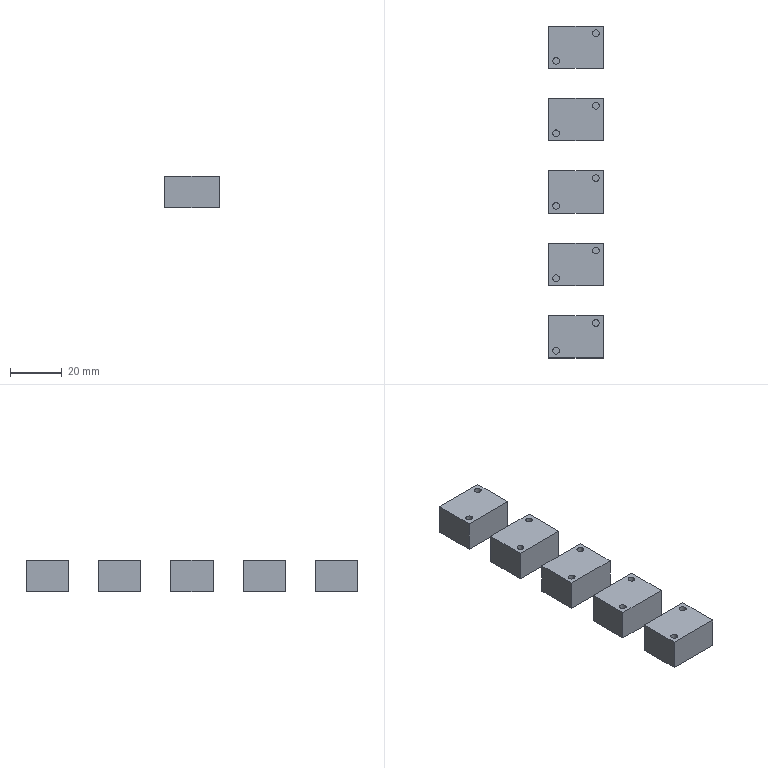Part | 5 solids | 60 faces | box 21 x 128.262 x 12 mm | volume 20066 mm3 | plane 40 | cylinder 20 | commonest cylinder face diameters 2.6 x20
STEP:
#1=CARTESIAN_POINT('',(-10.5,-47.869,0.));
#2=VERTEX_POINT('',#1);
#3=CARTESIAN_POINT('',(-10.5,-64.131,0.));
#4=VERTEX_POINT('',#3);
#5=CARTESIAN_POINT('',(-10.5,-47.869,0.));
#6=DIRECTION('',(0.,-1.,0.));
#7=VECTOR('',#6,1000.);
#8=LINE('',#5,#7);
#9=EDGE_CURVE('',#2,#4,#8,.T.);
#10=ORIENTED_EDGE('',*,*,#9,.T.);
#11=CARTESIAN_POINT('',(10.5,-64.131,0.));
#12=VERTEX_POINT('',#11);
#13=CARTESIAN_POINT('',(-10.5,-64.131,0.));
#14=DIRECTION('',(1.,0.,0.));
#15=VECTOR('',#14,1000.);
#16=LINE('',#13,#15);
#17=EDGE_CURVE('',#4,#12,#16,.T.);
#18=ORIENTED_EDGE('',*,*,#17,.T.);
#19=CARTESIAN_POINT('',(10.5,-47.869,0.));
#20=VERTEX_POINT('',#19);
#21=CARTESIAN_POINT('',(10.5,-64.131,0.));
#22=DIRECTION('',(0.,1.,0.));
#23=VECTOR('',#22,1000.);
#24=LINE('',#21,#23);
#25=EDGE_CURVE('',#12,#20,#24,.T.);
#26=ORIENTED_EDGE('',*,*,#25,.T.);
#27=CARTESIAN_POINT('',(10.5,-47.869,0.));
#28=DIRECTION('',(-1.,0.,0.));
#29=VECTOR('',#28,1000.);
#30=LINE('',#27,#29);
#31=EDGE_CURVE('',#20,#2,#30,.T.);
#32=ORIENTED_EDGE('',*,*,#31,.T.);
#33=EDGE_LOOP('',(#10,#18,#26,#32));
#34=FACE_BOUND('',#33,.T.);
#35=CARTESIAN_POINT('',(9.,-50.669,0.));
#36=VERTEX_POINT('',#35);
#37=CARTESIAN_POINT('',(6.4,-50.669,0.));
#38=VERTEX_POINT('',#37);
#39=CARTESIAN_POINT('',(7.7,-50.669,0.));
#40=DIRECTION('',(0.,0.,-1.));
#41=DIRECTION('',(1.,0.,0.));
#42=AXIS2_PLACEMENT_3D('',#39,#40,#41);
#43=CIRCLE('',#42,1.3);
#44=EDGE_CURVE('',#36,#38,#43,.T.);
#45=ORIENTED_EDGE('',*,*,#44,.T.);
#46=CARTESIAN_POINT('',(7.7,-50.669,0.));
#47=DIRECTION('',(0.,0.,-1.));
#48=DIRECTION('',(-1.,0.,0.));
#49=AXIS2_PLACEMENT_3D('',#46,#47,#48);
#50=CIRCLE('',#49,1.3);
#51=EDGE_CURVE('',#38,#36,#50,.T.);
#52=ORIENTED_EDGE('',*,*,#51,.T.);
#53=EDGE_LOOP('',(#45,#52));
#54=FACE_BOUND('',#53,.T.);
#55=CARTESIAN_POINT('',(-6.4,-61.331,0.));
#56=VERTEX_POINT('',#55);
#57=CARTESIAN_POINT('',(-9.,-61.331,0.));
#58=VERTEX_POINT('',#57);
#59=CARTESIAN_POINT('',(-7.7,-61.331,0.));
#60=DIRECTION('',(0.,0.,-1.));
#61=DIRECTION('',(1.,0.,0.));
#62=AXIS2_PLACEMENT_3D('',#59,#60,#61);
#63=CIRCLE('',#62,1.3);
#64=EDGE_CURVE('',#56,#58,#63,.T.);
#65=ORIENTED_EDGE('',*,*,#64,.T.);
#66=CARTESIAN_POINT('',(-7.7,-61.331,0.));
#67=DIRECTION('',(0.,0.,-1.));
#68=DIRECTION('',(-1.,0.,0.));
#69=AXIS2_PLACEMENT_3D('',#66,#67,#68);
#70=CIRCLE('',#69,1.3);
#71=EDGE_CURVE('',#58,#56,#70,.T.);
#72=ORIENTED_EDGE('',*,*,#71,.T.);
#73=EDGE_LOOP('',(#65,#72));
#74=FACE_BOUND('',#73,.T.);
#75=CARTESIAN_POINT('',(13.231,-129.333,0.));
#76=DIRECTION('',(0.,0.,-1.));
#77=DIRECTION('',(1.,0.,0.));
#78=AXIS2_PLACEMENT_3D('',#75,#76,#77);
#79=PLANE('',#78);
#80=ADVANCED_FACE('',(#34,#54,#74),#79,.F.);
#81=ORIENTED_EDGE('',*,*,#31,.F.);
#82=CARTESIAN_POINT('',(10.5,-47.869,-12.));
#83=VERTEX_POINT('',#82);
#84=CARTESIAN_POINT('',(10.5,-47.869,0.));
#85=DIRECTION('',(0.,0.,-1.));
#86=VECTOR('',#85,1000.);
#87=LINE('',#84,#86);
#88=EDGE_CURVE('',#20,#83,#87,.T.);
#89=ORIENTED_EDGE('',*,*,#88,.T.);
#90=CARTESIAN_POINT('',(-10.5,-47.869,-12.));
#91=VERTEX_POINT('',#90);
#92=CARTESIAN_POINT('',(10.5,-47.869,-12.));
#93=DIRECTION('',(-1.,0.,0.));
#94=VECTOR('',#93,1000.);
#95=LINE('',#92,#94);
#96=EDGE_CURVE('',#83,#91,#95,.T.);
#97=ORIENTED_EDGE('',*,*,#96,.T.);
#98=CARTESIAN_POINT('',(-10.5,-47.869,0.));
#99=DIRECTION('',(0.,0.,-1.));
#100=VECTOR('',#99,1000.);
#101=LINE('',#98,#100);
#102=EDGE_CURVE('',#2,#91,#101,.T.);
#103=ORIENTED_EDGE('',*,*,#102,.F.);
#104=EDGE_LOOP('',(#81,#89,#97,#103));
#105=FACE_BOUND('',#104,.T.);
#106=CARTESIAN_POINT('',(13.231,-47.869,0.));
#107=DIRECTION('',(0.,-1.,0.));
#108=DIRECTION('',(1.,0.,0.));
#109=AXIS2_PLACEMENT_3D('',#106,#107,#108);
#110=PLANE('',#109);
#111=ADVANCED_FACE('',(#105),#110,.F.);
#112=CARTESIAN_POINT('',(-10.5,-64.131,-12.));
#113=VERTEX_POINT('',#112);
#114=CARTESIAN_POINT('',(-10.5,-64.131,-12.));
#115=DIRECTION('',(0.,1.,0.));
#116=VECTOR('',#115,1000.);
#117=LINE('',#114,#116);
#118=EDGE_CURVE('',#113,#91,#117,.T.);
#119=ORIENTED_EDGE('',*,*,#118,.F.);
#120=CARTESIAN_POINT('',(-10.5,-64.131,-12.));
#121=DIRECTION('',(0.,0.,1.));
#122=VECTOR('',#121,1000.);
#123=LINE('',#120,#122);
#124=EDGE_CURVE('',#113,#4,#123,.T.);
#125=ORIENTED_EDGE('',*,*,#124,.T.);
#126=ORIENTED_EDGE('',*,*,#9,.F.);
#127=ORIENTED_EDGE('',*,*,#102,.T.);
#128=EDGE_LOOP('',(#119,#125,#126,#127));
#129=FACE_BOUND('',#128,.T.);
#130=CARTESIAN_POINT('',(-10.5,-64.131,0.));
#131=DIRECTION('',(-1.,0.,0.));
#132=DIRECTION('',(0.,-1.,0.));
#133=AXIS2_PLACEMENT_3D('',#130,#131,#132);
#134=PLANE('',#133);
#135=ADVANCED_FACE('',(#129),#134,.T.);
#136=ORIENTED_EDGE('',*,*,#124,.F.);
#137=CARTESIAN_POINT('',(10.5,-64.131,-12.));
#138=VERTEX_POINT('',#137);
#139=CARTESIAN_POINT('',(10.5,-64.131,-12.));
#140=DIRECTION('',(-1.,0.,0.));
#141=VECTOR('',#140,1000.);
#142=LINE('',#139,#141);
#143=EDGE_CURVE('',#138,#113,#142,.T.);
#144=ORIENTED_EDGE('',*,*,#143,.F.);
#145=CARTESIAN_POINT('',(10.5,-64.131,-12.));
#146=DIRECTION('',(0.,0.,1.));
#147=VECTOR('',#146,1000.);
#148=LINE('',#145,#147);
#149=EDGE_CURVE('',#138,#12,#148,.T.);
#150=ORIENTED_EDGE('',*,*,#149,.T.);
#151=ORIENTED_EDGE('',*,*,#17,.F.);
#152=EDGE_LOOP('',(#136,#144,#150,#151));
#153=FACE_BOUND('',#152,.T.);
#154=CARTESIAN_POINT('',(10.5,-64.131,0.));
#155=DIRECTION('',(0.,-1.,0.));
#156=DIRECTION('',(1.,0.,0.));
#157=AXIS2_PLACEMENT_3D('',#154,#155,#156);
#158=PLANE('',#157);
#159=ADVANCED_FACE('',(#153),#158,.T.);
#160=ORIENTED_EDGE('',*,*,#25,.F.);
#161=ORIENTED_EDGE('',*,*,#149,.F.);
#162=CARTESIAN_POINT('',(10.5,-47.869,-12.));
#163=DIRECTION('',(0.,-1.,0.));
#164=VECTOR('',#163,1000.);
#165=LINE('',#162,#164);
#166=EDGE_CURVE('',#83,#138,#165,.T.);
#167=ORIENTED_EDGE('',*,*,#166,.F.);
#168=ORIENTED_EDGE('',*,*,#88,.F.);
#169=EDGE_LOOP('',(#160,#161,#167,#168));
#170=FACE_BOUND('',#169,.T.);
#171=CARTESIAN_POINT('',(10.5,-43.561,0.));
#172=DIRECTION('',(1.,0.,0.));
#173=DIRECTION('',(0.,1.,0.));
#174=AXIS2_PLACEMENT_3D('',#171,#172,#173);
#175=PLANE('',#174);
#176=ADVANCED_FACE('',(#170),#175,.T.);
#177=ORIENTED_EDGE('',*,*,#166,.T.);
#178=ORIENTED_EDGE('',*,*,#143,.T.);
#179=ORIENTED_EDGE('',*,*,#118,.T.);
#180=ORIENTED_EDGE('',*,*,#96,.F.);
#181=EDGE_LOOP('',(#177,#178,#179,#180));
#182=FACE_BOUND('',#181,.T.);
#183=CARTESIAN_POINT('',(18.713,-139.577,-12.));
#184=DIRECTION('',(0.,0.,-1.));
#185=DIRECTION('',(1.,0.,0.));
#186=AXIS2_PLACEMENT_3D('',#183,#184,#185);
#187=PLANE('',#186);
#188=ADVANCED_FACE('',(#182),#187,.T.);
#189=CARTESIAN_POINT('',(6.4,-50.669,-8.));
#190=VERTEX_POINT('',#189);
#191=CARTESIAN_POINT('',(6.4,-50.669,0.));
#192=DIRECTION('',(0.,0.,-1.));
#193=VECTOR('',#192,1000.);
#194=LINE('',#191,#193);
#195=EDGE_CURVE('',#190,#38,#194,.F.);
#196=ORIENTED_EDGE('',*,*,#195,.F.);
#197=CARTESIAN_POINT('',(9.,-50.669,-8.));
#198=VERTEX_POINT('',#197);
#199=CARTESIAN_POINT('',(7.7,-50.669,-8.));
#200=DIRECTION('',(0.,0.,-1.));
#201=DIRECTION('',(-1.,0.,0.));
#202=AXIS2_PLACEMENT_3D('',#199,#200,#201);
#203=CIRCLE('',#202,1.3);
#204=EDGE_CURVE('',#190,#198,#203,.T.);
#205=ORIENTED_EDGE('',*,*,#204,.T.);
#206=CARTESIAN_POINT('',(9.,-50.669,0.));
#207=DIRECTION('',(0.,0.,-1.));
#208=VECTOR('',#207,1000.);
#209=LINE('',#206,#208);
#210=EDGE_CURVE('',#198,#36,#209,.F.);
#211=ORIENTED_EDGE('',*,*,#210,.T.);
#212=ORIENTED_EDGE('',*,*,#51,.F.);
#213=EDGE_LOOP('',(#196,#205,#211,#212));
#214=FACE_BOUND('',#213,.T.);
#215=CARTESIAN_POINT('',(7.7,-50.669,0.));
#216=DIRECTION('',(0.,0.,-1.));
#217=DIRECTION('',(1.,0.,0.));
#218=AXIS2_PLACEMENT_3D('',#215,#216,#217);
#219=CYLINDRICAL_SURFACE('',#218,1.3);
#220=ADVANCED_FACE('',(#214),#219,.F.);
#221=ORIENTED_EDGE('',*,*,#210,.F.);
#222=CARTESIAN_POINT('',(7.7,-50.669,-8.));
#223=DIRECTION('',(0.,0.,-1.));
#224=DIRECTION('',(1.,0.,0.));
#225=AXIS2_PLACEMENT_3D('',#222,#223,#224);
#226=CIRCLE('',#225,1.3);
#227=EDGE_CURVE('',#198,#190,#226,.T.);
#228=ORIENTED_EDGE('',*,*,#227,.T.);
#229=ORIENTED_EDGE('',*,*,#195,.T.);
#230=ORIENTED_EDGE('',*,*,#44,.F.);
#231=EDGE_LOOP('',(#221,#228,#229,#230));
#232=FACE_BOUND('',#231,.T.);
#233=CARTESIAN_POINT('',(7.7,-50.669,0.));
#234=DIRECTION('',(0.,0.,-1.));
#235=DIRECTION('',(1.,0.,0.));
#236=AXIS2_PLACEMENT_3D('',#233,#234,#235);
#237=CYLINDRICAL_SURFACE('',#236,1.3);
#238=ADVANCED_FACE('',(#232),#237,.F.);
#239=ORIENTED_EDGE('',*,*,#227,.F.);
#240=ORIENTED_EDGE('',*,*,#204,.F.);
#241=EDGE_LOOP('',(#239,#240));
#242=FACE_BOUND('',#241,.T.);
#243=CARTESIAN_POINT('',(13.231,-129.333,-8.));
#244=DIRECTION('',(0.,0.,-1.));
#245=DIRECTION('',(1.,0.,0.));
#246=AXIS2_PLACEMENT_3D('',#243,#244,#245);
#247=PLANE('',#246);
#248=ADVANCED_FACE('',(#242),#247,.F.);
#249=CARTESIAN_POINT('',(-6.4,-61.331,-8.));
#250=VERTEX_POINT('',#249);
#251=CARTESIAN_POINT('',(-9.,-61.331,-8.));
#252=VERTEX_POINT('',#251);
#253=CARTESIAN_POINT('',(-7.7,-61.331,-8.));
#254=DIRECTION('',(0.,0.,-1.));
#255=DIRECTION('',(1.,0.,0.));
#256=AXIS2_PLACEMENT_3D('',#253,#254,#255);
#257=CIRCLE('',#256,1.3);
#258=EDGE_CURVE('',#250,#252,#257,.T.);
#259=ORIENTED_EDGE('',*,*,#258,.F.);
#260=CARTESIAN_POINT('',(-7.7,-61.331,-8.));
#261=DIRECTION('',(0.,0.,-1.));
#262=DIRECTION('',(-1.,0.,0.));
#263=AXIS2_PLACEMENT_3D('',#260,#261,#262);
#264=CIRCLE('',#263,1.3);
#265=EDGE_CURVE('',#252,#250,#264,.T.);
#266=ORIENTED_EDGE('',*,*,#265,.F.);
#267=EDGE_LOOP('',(#259,#266));
#268=FACE_BOUND('',#267,.T.);
#269=CARTESIAN_POINT('',(13.231,-129.333,-8.));
#270=DIRECTION('',(0.,0.,-1.));
#271=DIRECTION('',(1.,0.,0.));
#272=AXIS2_PLACEMENT_3D('',#269,#270,#271);
#273=PLANE('',#272);
#274=ADVANCED_FACE('',(#268),#273,.F.);
#275=CARTESIAN_POINT('',(-9.,-61.331,0.));
#276=DIRECTION('',(0.,0.,-1.));
#277=VECTOR('',#276,1000.);
#278=LINE('',#275,#277);
#279=EDGE_CURVE('',#252,#58,#278,.F.);
#280=ORIENTED_EDGE('',*,*,#279,.F.);
#281=ORIENTED_EDGE('',*,*,#265,.T.);
#282=CARTESIAN_POINT('',(-6.4,-61.331,0.));
#283=DIRECTION('',(0.,0.,-1.));
#284=VECTOR('',#283,1000.);
#285=LINE('',#282,#284);
#286=EDGE_CURVE('',#250,#56,#285,.F.);
#287=ORIENTED_EDGE('',*,*,#286,.T.);
#288=ORIENTED_EDGE('',*,*,#71,.F.);
#289=EDGE_LOOP('',(#280,#281,#287,#288));
#290=FACE_BOUND('',#289,.T.);
#291=CARTESIAN_POINT('',(-7.7,-61.331,0.));
#292=DIRECTION('',(0.,0.,-1.));
#293=DIRECTION('',(1.,0.,0.));
#294=AXIS2_PLACEMENT_3D('',#291,#292,#293);
#295=CYLINDRICAL_SURFACE('',#294,1.3);
#296=ADVANCED_FACE('',(#290),#295,.F.);
#297=ORIENTED_EDGE('',*,*,#286,.F.);
#298=ORIENTED_EDGE('',*,*,#258,.T.);
#299=ORIENTED_EDGE('',*,*,#279,.T.);
#300=ORIENTED_EDGE('',*,*,#64,.F.);
#301=EDGE_LOOP('',(#297,#298,#299,#300));
#302=FACE_BOUND('',#301,.T.);
#303=CARTESIAN_POINT('',(-7.7,-61.331,0.));
#304=DIRECTION('',(0.,0.,-1.));
#305=DIRECTION('',(1.,0.,0.));
#306=AXIS2_PLACEMENT_3D('',#303,#304,#305);
#307=CYLINDRICAL_SURFACE('',#306,1.3);
#308=ADVANCED_FACE('',(#302),#307,.F.);
#309=CLOSED_SHELL('',(#80,#111,#135,#159,#176,#188,#220,#238,#248,#274,#296,#308));
#310=MANIFOLD_SOLID_BREP('',#309);
#311=CARTESIAN_POINT('',(-10.5,-19.869,0.));
#312=VERTEX_POINT('',#311);
#313=CARTESIAN_POINT('',(-10.5,-36.131,0.));
#314=VERTEX_POINT('',#313);
#315=CARTESIAN_POINT('',(-10.5,-19.869,0.));
#316=DIRECTION('',(0.,-1.,0.));
#317=VECTOR('',#316,1000.);
#318=LINE('',#315,#317);
#319=EDGE_CURVE('',#312,#314,#318,.T.);
#320=ORIENTED_EDGE('',*,*,#319,.T.);
#321=CARTESIAN_POINT('',(10.5,-36.131,0.));
#322=VERTEX_POINT('',#321);
#323=CARTESIAN_POINT('',(-10.5,-36.131,0.));
#324=DIRECTION('',(1.,0.,0.));
#325=VECTOR('',#324,1000.);
#326=LINE('',#323,#325);
#327=EDGE_CURVE('',#314,#322,#326,.T.);
#328=ORIENTED_EDGE('',*,*,#327,.T.);
#329=CARTESIAN_POINT('',(10.5,-19.869,0.));
#330=VERTEX_POINT('',#329);
#331=CARTESIAN_POINT('',(10.5,-36.131,0.));
#332=DIRECTION('',(0.,1.,0.));
#333=VECTOR('',#332,1000.);
#334=LINE('',#331,#333);
#335=EDGE_CURVE('',#322,#330,#334,.T.);
#336=ORIENTED_EDGE('',*,*,#335,.T.);
#337=CARTESIAN_POINT('',(10.5,-19.869,0.));
#338=DIRECTION('',(-1.,0.,0.));
#339=VECTOR('',#338,1000.);
#340=LINE('',#337,#339);
#341=EDGE_CURVE('',#330,#312,#340,.T.);
#342=ORIENTED_EDGE('',*,*,#341,.T.);
#343=EDGE_LOOP('',(#320,#328,#336,#342));
#344=FACE_BOUND('',#343,.T.);
#345=CARTESIAN_POINT('',(9.,-22.669,0.));
#346=VERTEX_POINT('',#345);
#347=CARTESIAN_POINT('',(6.4,-22.669,0.));
#348=VERTEX_POINT('',#347);
#349=CARTESIAN_POINT('',(7.7,-22.669,0.));
#350=DIRECTION('',(0.,0.,-1.));
#351=DIRECTION('',(1.,0.,0.));
#352=AXIS2_PLACEMENT_3D('',#349,#350,#351);
#353=CIRCLE('',#352,1.3);
#354=EDGE_CURVE('',#346,#348,#353,.T.);
#355=ORIENTED_EDGE('',*,*,#354,.T.);
#356=CARTESIAN_POINT('',(7.7,-22.669,0.));
#357=DIRECTION('',(0.,0.,-1.));
#358=DIRECTION('',(-1.,0.,0.));
#359=AXIS2_PLACEMENT_3D('',#356,#357,#358);
#360=CIRCLE('',#359,1.3);
#361=EDGE_CURVE('',#348,#346,#360,.T.);
#362=ORIENTED_EDGE('',*,*,#361,.T.);
#363=EDGE_LOOP('',(#355,#362));
#364=FACE_BOUND('',#363,.T.);
#365=CARTESIAN_POINT('',(-6.4,-33.331,0.));
#366=VERTEX_POINT('',#365);
#367=CARTESIAN_POINT('',(-9.,-33.331,0.));
#368=VERTEX_POINT('',#367);
#369=CARTESIAN_POINT('',(-7.7,-33.331,0.));
#370=DIRECTION('',(0.,0.,-1.));
#371=DIRECTION('',(1.,0.,0.));
#372=AXIS2_PLACEMENT_3D('',#369,#370,#371);
#373=CIRCLE('',#372,1.3);
#374=EDGE_CURVE('',#366,#368,#373,.T.);
#375=ORIENTED_EDGE('',*,*,#374,.T.);
#376=CARTESIAN_POINT('',(-7.7,-33.331,0.));
#377=DIRECTION('',(0.,0.,-1.));
#378=DIRECTION('',(-1.,0.,0.));
#379=AXIS2_PLACEMENT_3D('',#376,#377,#378);
#380=CIRCLE('',#379,1.3);
#381=EDGE_CURVE('',#368,#366,#380,.T.);
#382=ORIENTED_EDGE('',*,*,#381,.T.);
#383=EDGE_LOOP('',(#375,#382));
#384=FACE_BOUND('',#383,.T.);
#385=CARTESIAN_POINT('',(13.231,-101.333,0.));
#386=DIRECTION('',(0.,0.,-1.));
#387=DIRECTION('',(1.,0.,0.));
#388=AXIS2_PLACEMENT_3D('',#385,#386,#387);
#389=PLANE('',#388);
#390=ADVANCED_FACE('',(#344,#364,#384),#389,.F.);
#391=ORIENTED_EDGE('',*,*,#341,.F.);
#392=CARTESIAN_POINT('',(10.5,-19.869,-12.));
#393=VERTEX_POINT('',#392);
#394=CARTESIAN_POINT('',(10.5,-19.869,0.));
#395=DIRECTION('',(0.,0.,-1.));
#396=VECTOR('',#395,1000.);
#397=LINE('',#394,#396);
#398=EDGE_CURVE('',#330,#393,#397,.T.);
#399=ORIENTED_EDGE('',*,*,#398,.T.);
#400=CARTESIAN_POINT('',(-10.5,-19.869,-12.));
#401=VERTEX_POINT('',#400);
#402=CARTESIAN_POINT('',(10.5,-19.869,-12.));
#403=DIRECTION('',(-1.,0.,0.));
#404=VECTOR('',#403,1000.);
#405=LINE('',#402,#404);
#406=EDGE_CURVE('',#393,#401,#405,.T.);
#407=ORIENTED_EDGE('',*,*,#406,.T.);
#408=CARTESIAN_POINT('',(-10.5,-19.869,0.));
#409=DIRECTION('',(0.,0.,-1.));
#410=VECTOR('',#409,1000.);
#411=LINE('',#408,#410);
#412=EDGE_CURVE('',#312,#401,#411,.T.);
#413=ORIENTED_EDGE('',*,*,#412,.F.);
#414=EDGE_LOOP('',(#391,#399,#407,#413));
#415=FACE_BOUND('',#414,.T.);
#416=CARTESIAN_POINT('',(13.231,-19.869,0.));
#417=DIRECTION('',(0.,-1.,0.));
#418=DIRECTION('',(1.,0.,0.));
#419=AXIS2_PLACEMENT_3D('',#416,#417,#418);
#420=PLANE('',#419);
#421=ADVANCED_FACE('',(#415),#420,.F.);
#422=CARTESIAN_POINT('',(-10.5,-36.131,-12.));
#423=VERTEX_POINT('',#422);
#424=CARTESIAN_POINT('',(-10.5,-36.131,-12.));
#425=DIRECTION('',(0.,1.,0.));
#426=VECTOR('',#425,1000.);
#427=LINE('',#424,#426);
#428=EDGE_CURVE('',#423,#401,#427,.T.);
#429=ORIENTED_EDGE('',*,*,#428,.F.);
#430=CARTESIAN_POINT('',(-10.5,-36.131,-12.));
#431=DIRECTION('',(0.,0.,1.));
#432=VECTOR('',#431,1000.);
#433=LINE('',#430,#432);
#434=EDGE_CURVE('',#423,#314,#433,.T.);
#435=ORIENTED_EDGE('',*,*,#434,.T.);
#436=ORIENTED_EDGE('',*,*,#319,.F.);
#437=ORIENTED_EDGE('',*,*,#412,.T.);
#438=EDGE_LOOP('',(#429,#435,#436,#437));
#439=FACE_BOUND('',#438,.T.);
#440=CARTESIAN_POINT('',(-10.5,-36.131,0.));
#441=DIRECTION('',(-1.,0.,0.));
#442=DIRECTION('',(0.,-1.,0.));
#443=AXIS2_PLACEMENT_3D('',#440,#441,#442);
#444=PLANE('',#443);
#445=ADVANCED_FACE('',(#439),#444,.T.);
#446=ORIENTED_EDGE('',*,*,#434,.F.);
#447=CARTESIAN_POINT('',(10.5,-36.131,-12.));
#448=VERTEX_POINT('',#447);
#449=CARTESIAN_POINT('',(10.5,-36.131,-12.));
#450=DIRECTION('',(-1.,0.,0.));
#451=VECTOR('',#450,1000.);
#452=LINE('',#449,#451);
#453=EDGE_CURVE('',#448,#423,#452,.T.);
#454=ORIENTED_EDGE('',*,*,#453,.F.);
#455=CARTESIAN_POINT('',(10.5,-36.131,-12.));
#456=DIRECTION('',(0.,0.,1.));
#457=VECTOR('',#456,1000.);
#458=LINE('',#455,#457);
#459=EDGE_CURVE('',#448,#322,#458,.T.);
#460=ORIENTED_EDGE('',*,*,#459,.T.);
#461=ORIENTED_EDGE('',*,*,#327,.F.);
#462=EDGE_LOOP('',(#446,#454,#460,#461));
#463=FACE_BOUND('',#462,.T.);
#464=CARTESIAN_POINT('',(10.5,-36.131,0.));
#465=DIRECTION('',(0.,-1.,0.));
#466=DIRECTION('',(1.,0.,0.));
#467=AXIS2_PLACEMENT_3D('',#464,#465,#466);
#468=PLANE('',#467);
#469=ADVANCED_FACE('',(#463),#468,.T.);
#470=ORIENTED_EDGE('',*,*,#335,.F.);
#471=ORIENTED_EDGE('',*,*,#459,.F.);
#472=CARTESIAN_POINT('',(10.5,-19.869,-12.));
#473=DIRECTION('',(0.,-1.,0.));
#474=VECTOR('',#473,1000.);
#475=LINE('',#472,#474);
#476=EDGE_CURVE('',#393,#448,#475,.T.);
#477=ORIENTED_EDGE('',*,*,#476,.F.);
#478=ORIENTED_EDGE('',*,*,#398,.F.);
#479=EDGE_LOOP('',(#470,#471,#477,#478));
#480=FACE_BOUND('',#479,.T.);
#481=CARTESIAN_POINT('',(10.5,-15.561,0.));
#482=DIRECTION('',(1.,0.,0.));
#483=DIRECTION('',(0.,1.,0.));
#484=AXIS2_PLACEMENT_3D('',#481,#482,#483);
#485=PLANE('',#484);
#486=ADVANCED_FACE('',(#480),#485,.T.);
#487=ORIENTED_EDGE('',*,*,#476,.T.);
#488=ORIENTED_EDGE('',*,*,#453,.T.);
#489=ORIENTED_EDGE('',*,*,#428,.T.);
#490=ORIENTED_EDGE('',*,*,#406,.F.);
#491=EDGE_LOOP('',(#487,#488,#489,#490));
#492=FACE_BOUND('',#491,.T.);
#493=CARTESIAN_POINT('',(18.713,-111.577,-12.));
#494=DIRECTION('',(0.,0.,-1.));
#495=DIRECTION('',(1.,0.,0.));
#496=AXIS2_PLACEMENT_3D('',#493,#494,#495);
#497=PLANE('',#496);
#498=ADVANCED_FACE('',(#492),#497,.T.);
#499=CARTESIAN_POINT('',(6.4,-22.669,-8.));
#500=VERTEX_POINT('',#499);
#501=CARTESIAN_POINT('',(6.4,-22.669,0.));
#502=DIRECTION('',(0.,0.,-1.));
#503=VECTOR('',#502,1000.);
#504=LINE('',#501,#503);
#505=EDGE_CURVE('',#500,#348,#504,.F.);
#506=ORIENTED_EDGE('',*,*,#505,.F.);
#507=CARTESIAN_POINT('',(9.,-22.669,-8.));
#508=VERTEX_POINT('',#507);
#509=CARTESIAN_POINT('',(7.7,-22.669,-8.));
#510=DIRECTION('',(0.,0.,-1.));
#511=DIRECTION('',(-1.,0.,0.));
#512=AXIS2_PLACEMENT_3D('',#509,#510,#511);
#513=CIRCLE('',#512,1.3);
#514=EDGE_CURVE('',#500,#508,#513,.T.);
#515=ORIENTED_EDGE('',*,*,#514,.T.);
#516=CARTESIAN_POINT('',(9.,-22.669,0.));
#517=DIRECTION('',(0.,0.,-1.));
#518=VECTOR('',#517,1000.);
#519=LINE('',#516,#518);
#520=EDGE_CURVE('',#508,#346,#519,.F.);
#521=ORIENTED_EDGE('',*,*,#520,.T.);
#522=ORIENTED_EDGE('',*,*,#361,.F.);
#523=EDGE_LOOP('',(#506,#515,#521,#522));
#524=FACE_BOUND('',#523,.T.);
#525=CARTESIAN_POINT('',(7.7,-22.669,0.));
#526=DIRECTION('',(0.,0.,-1.));
#527=DIRECTION('',(1.,0.,0.));
#528=AXIS2_PLACEMENT_3D('',#525,#526,#527);
#529=CYLINDRICAL_SURFACE('',#528,1.3);
#530=ADVANCED_FACE('',(#524),#529,.F.);
#531=ORIENTED_EDGE('',*,*,#520,.F.);
#532=CARTESIAN_POINT('',(7.7,-22.669,-8.));
#533=DIRECTION('',(0.,0.,-1.));
#534=DIRECTION('',(1.,0.,0.));
#535=AXIS2_PLACEMENT_3D('',#532,#533,#534);
#536=CIRCLE('',#535,1.3);
#537=EDGE_CURVE('',#508,#500,#536,.T.);
#538=ORIENTED_EDGE('',*,*,#537,.T.);
#539=ORIENTED_EDGE('',*,*,#505,.T.);
#540=ORIENTED_EDGE('',*,*,#354,.F.);
#541=EDGE_LOOP('',(#531,#538,#539,#540));
#542=FACE_BOUND('',#541,.T.);
#543=CARTESIAN_POINT('',(7.7,-22.669,0.));
#544=DIRECTION('',(0.,0.,-1.));
#545=DIRECTION('',(1.,0.,0.));
#546=AXIS2_PLACEMENT_3D('',#543,#544,#545);
#547=CYLINDRICAL_SURFACE('',#546,1.3);
#548=ADVANCED_FACE('',(#542),#547,.F.);
#549=ORIENTED_EDGE('',*,*,#537,.F.);
#550=ORIENTED_EDGE('',*,*,#514,.F.);
#551=EDGE_LOOP('',(#549,#550));
#552=FACE_BOUND('',#551,.T.);
#553=CARTESIAN_POINT('',(13.231,-101.333,-8.));
#554=DIRECTION('',(0.,0.,-1.));
#555=DIRECTION('',(1.,0.,0.));
#556=AXIS2_PLACEMENT_3D('',#553,#554,#555);
#557=PLANE('',#556);
#558=ADVANCED_FACE('',(#552),#557,.F.);
#559=CARTESIAN_POINT('',(-6.4,-33.331,-8.));
#560=VERTEX_POINT('',#559);
#561=CARTESIAN_POINT('',(-9.,-33.331,-8.));
#562=VERTEX_POINT('',#561);
#563=CARTESIAN_POINT('',(-7.7,-33.331,-8.));
#564=DIRECTION('',(0.,0.,-1.));
#565=DIRECTION('',(1.,0.,0.));
#566=AXIS2_PLACEMENT_3D('',#563,#564,#565);
#567=CIRCLE('',#566,1.3);
#568=EDGE_CURVE('',#560,#562,#567,.T.);
#569=ORIENTED_EDGE('',*,*,#568,.F.);
#570=CARTESIAN_POINT('',(-7.7,-33.331,-8.));
#571=DIRECTION('',(0.,0.,-1.));
#572=DIRECTION('',(-1.,0.,0.));
#573=AXIS2_PLACEMENT_3D('',#570,#571,#572);
#574=CIRCLE('',#573,1.3);
#575=EDGE_CURVE('',#562,#560,#574,.T.);
#576=ORIENTED_EDGE('',*,*,#575,.F.);
#577=EDGE_LOOP('',(#569,#576));
#578=FACE_BOUND('',#577,.T.);
#579=CARTESIAN_POINT('',(13.231,-101.333,-8.));
#580=DIRECTION('',(0.,0.,-1.));
#581=DIRECTION('',(1.,0.,0.));
#582=AXIS2_PLACEMENT_3D('',#579,#580,#581);
#583=PLANE('',#582);
#584=ADVANCED_FACE('',(#578),#583,.F.);
#585=CARTESIAN_POINT('',(-9.,-33.331,0.));
#586=DIRECTION('',(0.,0.,-1.));
#587=VECTOR('',#586,1000.);
#588=LINE('',#585,#587);
#589=EDGE_CURVE('',#562,#368,#588,.F.);
#590=ORIENTED_EDGE('',*,*,#589,.F.);
#591=ORIENTED_EDGE('',*,*,#575,.T.);
#592=CARTESIAN_POINT('',(-6.4,-33.331,0.));
#593=DIRECTION('',(0.,0.,-1.));
#594=VECTOR('',#593,1000.);
#595=LINE('',#592,#594);
#596=EDGE_CURVE('',#560,#366,#595,.F.);
#597=ORIENTED_EDGE('',*,*,#596,.T.);
#598=ORIENTED_EDGE('',*,*,#381,.F.);
#599=EDGE_LOOP('',(#590,#591,#597,#598));
#600=FACE_BOUND('',#599,.T.);
#601=CARTESIAN_POINT('',(-7.7,-33.331,0.));
#602=DIRECTION('',(0.,0.,-1.));
#603=DIRECTION('',(1.,0.,0.));
#604=AXIS2_PLACEMENT_3D('',#601,#602,#603);
#605=CYLINDRICAL_SURFACE('',#604,1.3);
#606=ADVANCED_FACE('',(#600),#605,.F.);
#607=ORIENTED_EDGE('',*,*,#596,.F.);
#608=ORIENTED_EDGE('',*,*,#568,.T.);
#609=ORIENTED_EDGE('',*,*,#589,.T.);
#610=ORIENTED_EDGE('',*,*,#374,.F.);
#611=EDGE_LOOP('',(#607,#608,#609,#610));
#612=FACE_BOUND('',#611,.T.);
#613=CARTESIAN_POINT('',(-7.7,-33.331,0.));
#614=DIRECTION('',(0.,0.,-1.));
#615=DIRECTION('',(1.,0.,0.));
#616=AXIS2_PLACEMENT_3D('',#613,#614,#615);
#617=CYLINDRICAL_SURFACE('',#616,1.3);
#618=ADVANCED_FACE('',(#612),#617,.F.);
#619=CLOSED_SHELL('',(#390,#421,#445,#469,#486,#498,#530,#548,#558,#584,#606,#618));
#620=MANIFOLD_SOLID_BREP('',#619);
#621=CARTESIAN_POINT('',(-10.5,-103.869,0.));
#622=VERTEX_POINT('',#621);
#623=CARTESIAN_POINT('',(-10.5,-120.131,0.));
#624=VERTEX_POINT('',#623);
#625=CARTESIAN_POINT('',(-10.5,-103.869,0.));
#626=DIRECTION('',(0.,-1.,0.));
#627=VECTOR('',#626,1000.);
#628=LINE('',#625,#627);
#629=EDGE_CURVE('',#622,#624,#628,.T.);
#630=ORIENTED_EDGE('',*,*,#629,.T.);
#631=CARTESIAN_POINT('',(10.5,-120.131,0.));
#632=VERTEX_POINT('',#631);
#633=CARTESIAN_POINT('',(-10.5,-120.131,0.));
#634=DIRECTION('',(1.,0.,0.));
#635=VECTOR('',#634,1000.);
#636=LINE('',#633,#635);
#637=EDGE_CURVE('',#624,#632,#636,.T.);
#638=ORIENTED_EDGE('',*,*,#637,.T.);
#639=CARTESIAN_POINT('',(10.5,-103.869,0.));
#640=VERTEX_POINT('',#639);
#641=CARTESIAN_POINT('',(10.5,-120.131,0.));
#642=DIRECTION('',(0.,1.,0.));
#643=VECTOR('',#642,1000.);
#644=LINE('',#641,#643);
#645=EDGE_CURVE('',#632,#640,#644,.T.);
#646=ORIENTED_EDGE('',*,*,#645,.T.);
#647=CARTESIAN_POINT('',(10.5,-103.869,0.));
#648=DIRECTION('',(-1.,0.,0.));
#649=VECTOR('',#648,1000.);
#650=LINE('',#647,#649);
#651=EDGE_CURVE('',#640,#622,#650,.T.);
#652=ORIENTED_EDGE('',*,*,#651,.T.);
#653=EDGE_LOOP('',(#630,#638,#646,#652));
#654=FACE_BOUND('',#653,.T.);
#655=CARTESIAN_POINT('',(9.,-106.669,0.));
#656=VERTEX_POINT('',#655);
#657=CARTESIAN_POINT('',(6.4,-106.669,0.));
#658=VERTEX_POINT('',#657);
#659=CARTESIAN_POINT('',(7.7,-106.669,0.));
#660=DIRECTION('',(0.,0.,-1.));
#661=DIRECTION('',(1.,0.,0.));
#662=AXIS2_PLACEMENT_3D('',#659,#660,#661);
#663=CIRCLE('',#662,1.3);
#664=EDGE_CURVE('',#656,#658,#663,.T.);
#665=ORIENTED_EDGE('',*,*,#664,.T.);
#666=CARTESIAN_POINT('',(7.7,-106.669,0.));
#667=DIRECTION('',(0.,0.,-1.));
#668=DIRECTION('',(-1.,0.,0.));
#669=AXIS2_PLACEMENT_3D('',#666,#667,#668);
#670=CIRCLE('',#669,1.3);
#671=EDGE_CURVE('',#658,#656,#670,.T.);
#672=ORIENTED_EDGE('',*,*,#671,.T.);
#673=EDGE_LOOP('',(#665,#672));
#674=FACE_BOUND('',#673,.T.);
#675=CARTESIAN_POINT('',(-6.4,-117.331,0.));
#676=VERTEX_POINT('',#675);
#677=CARTESIAN_POINT('',(-9.,-117.331,0.));
#678=VERTEX_POINT('',#677);
#679=CARTESIAN_POINT('',(-7.7,-117.331,0.));
#680=DIRECTION('',(0.,0.,-1.));
#681=DIRECTION('',(1.,0.,0.));
#682=AXIS2_PLACEMENT_3D('',#679,#680,#681);
#683=CIRCLE('',#682,1.3);
#684=EDGE_CURVE('',#676,#678,#683,.T.);
#685=ORIENTED_EDGE('',*,*,#684,.T.);
#686=CARTESIAN_POINT('',(-7.7,-117.331,0.));
#687=DIRECTION('',(0.,0.,-1.));
#688=DIRECTION('',(-1.,0.,0.));
#689=AXIS2_PLACEMENT_3D('',#686,#687,#688);
#690=CIRCLE('',#689,1.3);
#691=EDGE_CURVE('',#678,#676,#690,.T.);
#692=ORIENTED_EDGE('',*,*,#691,.T.);
#693=EDGE_LOOP('',(#685,#692));
#694=FACE_BOUND('',#693,.T.);
#695=CARTESIAN_POINT('',(13.231,-185.333,0.));
#696=DIRECTION('',(0.,0.,-1.));
#697=DIRECTION('',(1.,0.,0.));
#698=AXIS2_PLACEMENT_3D('',#695,#696,#697);
#699=PLANE('',#698);
#700=ADVANCED_FACE('',(#654,#674,#694),#699,.F.);
#701=ORIENTED_EDGE('',*,*,#651,.F.);
#702=CARTESIAN_POINT('',(10.5,-103.869,-12.));
#703=VERTEX_POINT('',#702);
#704=CARTESIAN_POINT('',(10.5,-103.869,0.));
#705=DIRECTION('',(0.,0.,-1.));
#706=VECTOR('',#705,1000.);
#707=LINE('',#704,#706);
#708=EDGE_CURVE('',#640,#703,#707,.T.);
#709=ORIENTED_EDGE('',*,*,#708,.T.);
#710=CARTESIAN_POINT('',(-10.5,-103.869,-12.));
#711=VERTEX_POINT('',#710);
#712=CARTESIAN_POINT('',(10.5,-103.869,-12.));
#713=DIRECTION('',(-1.,0.,0.));
#714=VECTOR('',#713,1000.);
#715=LINE('',#712,#714);
#716=EDGE_CURVE('',#703,#711,#715,.T.);
#717=ORIENTED_EDGE('',*,*,#716,.T.);
#718=CARTESIAN_POINT('',(-10.5,-103.869,0.));
#719=DIRECTION('',(0.,0.,-1.));
#720=VECTOR('',#719,1000.);
#721=LINE('',#718,#720);
#722=EDGE_CURVE('',#622,#711,#721,.T.);
#723=ORIENTED_EDGE('',*,*,#722,.F.);
#724=EDGE_LOOP('',(#701,#709,#717,#723));
#725=FACE_BOUND('',#724,.T.);
#726=CARTESIAN_POINT('',(13.231,-103.869,0.));
#727=DIRECTION('',(0.,-1.,0.));
#728=DIRECTION('',(1.,0.,0.));
#729=AXIS2_PLACEMENT_3D('',#726,#727,#728);
#730=PLANE('',#729);
#731=ADVANCED_FACE('',(#725),#730,.F.);
#732=CARTESIAN_POINT('',(-10.5,-120.131,-12.));
#733=VERTEX_POINT('',#732);
#734=CARTESIAN_POINT('',(-10.5,-120.131,-12.));
#735=DIRECTION('',(0.,1.,0.));
#736=VECTOR('',#735,1000.);
#737=LINE('',#734,#736);
#738=EDGE_CURVE('',#733,#711,#737,.T.);
#739=ORIENTED_EDGE('',*,*,#738,.F.);
#740=CARTESIAN_POINT('',(-10.5,-120.131,-12.));
#741=DIRECTION('',(0.,0.,1.));
#742=VECTOR('',#741,1000.);
#743=LINE('',#740,#742);
#744=EDGE_CURVE('',#733,#624,#743,.T.);
#745=ORIENTED_EDGE('',*,*,#744,.T.);
#746=ORIENTED_EDGE('',*,*,#629,.F.);
#747=ORIENTED_EDGE('',*,*,#722,.T.);
#748=EDGE_LOOP('',(#739,#745,#746,#747));
#749=FACE_BOUND('',#748,.T.);
#750=CARTESIAN_POINT('',(-10.5,-120.131,0.));
#751=DIRECTION('',(-1.,0.,0.));
#752=DIRECTION('',(0.,-1.,0.));
#753=AXIS2_PLACEMENT_3D('',#750,#751,#752);
#754=PLANE('',#753);
#755=ADVANCED_FACE('',(#749),#754,.T.);
#756=ORIENTED_EDGE('',*,*,#744,.F.);
#757=CARTESIAN_POINT('',(10.5,-120.131,-12.));
#758=VERTEX_POINT('',#757);
#759=CARTESIAN_POINT('',(10.5,-120.131,-12.));
#760=DIRECTION('',(-1.,0.,0.));
#761=VECTOR('',#760,1000.);
#762=LINE('',#759,#761);
#763=EDGE_CURVE('',#758,#733,#762,.T.);
#764=ORIENTED_EDGE('',*,*,#763,.F.);
#765=CARTESIAN_POINT('',(10.5,-120.131,-12.));
#766=DIRECTION('',(0.,0.,1.));
#767=VECTOR('',#766,1000.);
#768=LINE('',#765,#767);
#769=EDGE_CURVE('',#758,#632,#768,.T.);
#770=ORIENTED_EDGE('',*,*,#769,.T.);
#771=ORIENTED_EDGE('',*,*,#637,.F.);
#772=EDGE_LOOP('',(#756,#764,#770,#771));
#773=FACE_BOUND('',#772,.T.);
#774=CARTESIAN_POINT('',(10.5,-120.131,0.));
#775=DIRECTION('',(0.,-1.,0.));
#776=DIRECTION('',(1.,0.,0.));
#777=AXIS2_PLACEMENT_3D('',#774,#775,#776);
#778=PLANE('',#777);
#779=ADVANCED_FACE('',(#773),#778,.T.);
#780=ORIENTED_EDGE('',*,*,#645,.F.);
#781=ORIENTED_EDGE('',*,*,#769,.F.);
#782=CARTESIAN_POINT('',(10.5,-103.869,-12.));
#783=DIRECTION('',(0.,-1.,0.));
#784=VECTOR('',#783,1000.);
#785=LINE('',#782,#784);
#786=EDGE_CURVE('',#703,#758,#785,.T.);
#787=ORIENTED_EDGE('',*,*,#786,.F.);
#788=ORIENTED_EDGE('',*,*,#708,.F.);
#789=EDGE_LOOP('',(#780,#781,#787,#788));
#790=FACE_BOUND('',#789,.T.);
#791=CARTESIAN_POINT('',(10.5,-99.561,0.));
#792=DIRECTION('',(1.,0.,0.));
#793=DIRECTION('',(0.,1.,0.));
#794=AXIS2_PLACEMENT_3D('',#791,#792,#793);
#795=PLANE('',#794);
#796=ADVANCED_FACE('',(#790),#795,.T.);
#797=ORIENTED_EDGE('',*,*,#786,.T.);
#798=ORIENTED_EDGE('',*,*,#763,.T.);
#799=ORIENTED_EDGE('',*,*,#738,.T.);
#800=ORIENTED_EDGE('',*,*,#716,.F.);
#801=EDGE_LOOP('',(#797,#798,#799,#800));
#802=FACE_BOUND('',#801,.T.);
#803=CARTESIAN_POINT('',(18.713,-195.577,-12.));
#804=DIRECTION('',(0.,0.,-1.));
#805=DIRECTION('',(1.,0.,0.));
#806=AXIS2_PLACEMENT_3D('',#803,#804,#805);
#807=PLANE('',#806);
#808=ADVANCED_FACE('',(#802),#807,.T.);
#809=CARTESIAN_POINT('',(6.4,-106.669,-8.));
#810=VERTEX_POINT('',#809);
#811=CARTESIAN_POINT('',(6.4,-106.669,0.));
#812=DIRECTION('',(0.,0.,-1.));
#813=VECTOR('',#812,1000.);
#814=LINE('',#811,#813);
#815=EDGE_CURVE('',#810,#658,#814,.F.);
#816=ORIENTED_EDGE('',*,*,#815,.F.);
#817=CARTESIAN_POINT('',(9.,-106.669,-8.));
#818=VERTEX_POINT('',#817);
#819=CARTESIAN_POINT('',(7.7,-106.669,-8.));
#820=DIRECTION('',(0.,0.,-1.));
#821=DIRECTION('',(-1.,0.,0.));
#822=AXIS2_PLACEMENT_3D('',#819,#820,#821);
#823=CIRCLE('',#822,1.3);
#824=EDGE_CURVE('',#810,#818,#823,.T.);
#825=ORIENTED_EDGE('',*,*,#824,.T.);
#826=CARTESIAN_POINT('',(9.,-106.669,0.));
#827=DIRECTION('',(0.,0.,-1.));
#828=VECTOR('',#827,1000.);
#829=LINE('',#826,#828);
#830=EDGE_CURVE('',#818,#656,#829,.F.);
#831=ORIENTED_EDGE('',*,*,#830,.T.);
#832=ORIENTED_EDGE('',*,*,#671,.F.);
#833=EDGE_LOOP('',(#816,#825,#831,#832));
#834=FACE_BOUND('',#833,.T.);
#835=CARTESIAN_POINT('',(7.7,-106.669,0.));
#836=DIRECTION('',(0.,0.,-1.));
#837=DIRECTION('',(1.,0.,0.));
#838=AXIS2_PLACEMENT_3D('',#835,#836,#837);
#839=CYLINDRICAL_SURFACE('',#838,1.3);
#840=ADVANCED_FACE('',(#834),#839,.F.);
#841=ORIENTED_EDGE('',*,*,#830,.F.);
#842=CARTESIAN_POINT('',(7.7,-106.669,-8.));
#843=DIRECTION('',(0.,0.,-1.));
#844=DIRECTION('',(1.,0.,0.));
#845=AXIS2_PLACEMENT_3D('',#842,#843,#844);
#846=CIRCLE('',#845,1.3);
#847=EDGE_CURVE('',#818,#810,#846,.T.);
#848=ORIENTED_EDGE('',*,*,#847,.T.);
#849=ORIENTED_EDGE('',*,*,#815,.T.);
#850=ORIENTED_EDGE('',*,*,#664,.F.);
#851=EDGE_LOOP('',(#841,#848,#849,#850));
#852=FACE_BOUND('',#851,.T.);
#853=CARTESIAN_POINT('',(7.7,-106.669,0.));
#854=DIRECTION('',(0.,0.,-1.));
#855=DIRECTION('',(1.,0.,0.));
#856=AXIS2_PLACEMENT_3D('',#853,#854,#855);
#857=CYLINDRICAL_SURFACE('',#856,1.3);
#858=ADVANCED_FACE('',(#852),#857,.F.);
#859=ORIENTED_EDGE('',*,*,#847,.F.);
#860=ORIENTED_EDGE('',*,*,#824,.F.);
#861=EDGE_LOOP('',(#859,#860));
#862=FACE_BOUND('',#861,.T.);
#863=CARTESIAN_POINT('',(13.231,-185.333,-8.));
#864=DIRECTION('',(0.,0.,-1.));
#865=DIRECTION('',(1.,0.,0.));
#866=AXIS2_PLACEMENT_3D('',#863,#864,#865);
#867=PLANE('',#866);
#868=ADVANCED_FACE('',(#862),#867,.F.);
#869=CARTESIAN_POINT('',(-6.4,-117.331,-8.));
#870=VERTEX_POINT('',#869);
#871=CARTESIAN_POINT('',(-9.,-117.331,-8.));
#872=VERTEX_POINT('',#871);
#873=CARTESIAN_POINT('',(-7.7,-117.331,-8.));
#874=DIRECTION('',(0.,0.,-1.));
#875=DIRECTION('',(1.,0.,0.));
#876=AXIS2_PLACEMENT_3D('',#873,#874,#875);
#877=CIRCLE('',#876,1.3);
#878=EDGE_CURVE('',#870,#872,#877,.T.);
#879=ORIENTED_EDGE('',*,*,#878,.F.);
#880=CARTESIAN_POINT('',(-7.7,-117.331,-8.));
#881=DIRECTION('',(0.,0.,-1.));
#882=DIRECTION('',(-1.,0.,0.));
#883=AXIS2_PLACEMENT_3D('',#880,#881,#882);
#884=CIRCLE('',#883,1.3);
#885=EDGE_CURVE('',#872,#870,#884,.T.);
#886=ORIENTED_EDGE('',*,*,#885,.F.);
#887=EDGE_LOOP('',(#879,#886));
#888=FACE_BOUND('',#887,.T.);
#889=CARTESIAN_POINT('',(13.231,-185.333,-8.));
#890=DIRECTION('',(0.,0.,-1.));
#891=DIRECTION('',(1.,0.,0.));
#892=AXIS2_PLACEMENT_3D('',#889,#890,#891);
#893=PLANE('',#892);
#894=ADVANCED_FACE('',(#888),#893,.F.);
#895=CARTESIAN_POINT('',(-9.,-117.331,0.));
#896=DIRECTION('',(0.,0.,-1.));
#897=VECTOR('',#896,1000.);
#898=LINE('',#895,#897);
#899=EDGE_CURVE('',#872,#678,#898,.F.);
#900=ORIENTED_EDGE('',*,*,#899,.F.);
#901=ORIENTED_EDGE('',*,*,#885,.T.);
#902=CARTESIAN_POINT('',(-6.4,-117.331,0.));
#903=DIRECTION('',(0.,0.,-1.));
#904=VECTOR('',#903,1000.);
#905=LINE('',#902,#904);
#906=EDGE_CURVE('',#870,#676,#905,.F.);
#907=ORIENTED_EDGE('',*,*,#906,.T.);
#908=ORIENTED_EDGE('',*,*,#691,.F.);
#909=EDGE_LOOP('',(#900,#901,#907,#908));
#910=FACE_BOUND('',#909,.T.);
#911=CARTESIAN_POINT('',(-7.7,-117.331,0.));
#912=DIRECTION('',(0.,0.,-1.));
#913=DIRECTION('',(1.,0.,0.));
#914=AXIS2_PLACEMENT_3D('',#911,#912,#913);
#915=CYLINDRICAL_SURFACE('',#914,1.3);
#916=ADVANCED_FACE('',(#910),#915,.F.);
#917=ORIENTED_EDGE('',*,*,#906,.F.);
#918=ORIENTED_EDGE('',*,*,#878,.T.);
#919=ORIENTED_EDGE('',*,*,#899,.T.);
#920=ORIENTED_EDGE('',*,*,#684,.F.);
#921=EDGE_LOOP('',(#917,#918,#919,#920));
#922=FACE_BOUND('',#921,.T.);
#923=CARTESIAN_POINT('',(-7.7,-117.331,0.));
#924=DIRECTION('',(0.,0.,-1.));
#925=DIRECTION('',(1.,0.,0.));
#926=AXIS2_PLACEMENT_3D('',#923,#924,#925);
#927=CYLINDRICAL_SURFACE('',#926,1.3);
#928=ADVANCED_FACE('',(#922),#927,.F.);
#929=CLOSED_SHELL('',(#700,#731,#755,#779,#796,#808,#840,#858,#868,#894,#916,#928));
#930=MANIFOLD_SOLID_BREP('',#929);
#931=CARTESIAN_POINT('',(-10.5,-75.869,0.));
#932=VERTEX_POINT('',#931);
#933=CARTESIAN_POINT('',(-10.5,-92.131,0.));
#934=VERTEX_POINT('',#933);
#935=CARTESIAN_POINT('',(-10.5,-75.869,0.));
#936=DIRECTION('',(0.,-1.,0.));
#937=VECTOR('',#936,1000.);
#938=LINE('',#935,#937);
#939=EDGE_CURVE('',#932,#934,#938,.T.);
#940=ORIENTED_EDGE('',*,*,#939,.T.);
#941=CARTESIAN_POINT('',(10.5,-92.131,0.));
#942=VERTEX_POINT('',#941);
#943=CARTESIAN_POINT('',(-10.5,-92.131,0.));
#944=DIRECTION('',(1.,0.,0.));
#945=VECTOR('',#944,1000.);
#946=LINE('',#943,#945);
#947=EDGE_CURVE('',#934,#942,#946,.T.);
#948=ORIENTED_EDGE('',*,*,#947,.T.);
#949=CARTESIAN_POINT('',(10.5,-75.869,0.));
#950=VERTEX_POINT('',#949);
#951=CARTESIAN_POINT('',(10.5,-92.131,0.));
#952=DIRECTION('',(0.,1.,0.));
#953=VECTOR('',#952,1000.);
#954=LINE('',#951,#953);
#955=EDGE_CURVE('',#942,#950,#954,.T.);
#956=ORIENTED_EDGE('',*,*,#955,.T.);
#957=CARTESIAN_POINT('',(10.5,-75.869,0.));
#958=DIRECTION('',(-1.,0.,0.));
#959=VECTOR('',#958,1000.);
#960=LINE('',#957,#959);
#961=EDGE_CURVE('',#950,#932,#960,.T.);
#962=ORIENTED_EDGE('',*,*,#961,.T.);
#963=EDGE_LOOP('',(#940,#948,#956,#962));
#964=FACE_BOUND('',#963,.T.);
#965=CARTESIAN_POINT('',(9.,-78.669,0.));
#966=VERTEX_POINT('',#965);
#967=CARTESIAN_POINT('',(6.4,-78.669,0.));
#968=VERTEX_POINT('',#967);
#969=CARTESIAN_POINT('',(7.7,-78.669,0.));
#970=DIRECTION('',(0.,0.,-1.));
#971=DIRECTION('',(1.,0.,0.));
#972=AXIS2_PLACEMENT_3D('',#969,#970,#971);
#973=CIRCLE('',#972,1.3);
#974=EDGE_CURVE('',#966,#968,#973,.T.);
#975=ORIENTED_EDGE('',*,*,#974,.T.);
#976=CARTESIAN_POINT('',(7.7,-78.669,0.));
#977=DIRECTION('',(0.,0.,-1.));
#978=DIRECTION('',(-1.,0.,0.));
#979=AXIS2_PLACEMENT_3D('',#976,#977,#978);
#980=CIRCLE('',#979,1.3);
#981=EDGE_CURVE('',#968,#966,#980,.T.);
#982=ORIENTED_EDGE('',*,*,#981,.T.);
#983=EDGE_LOOP('',(#975,#982));
#984=FACE_BOUND('',#983,.T.);
#985=CARTESIAN_POINT('',(-6.4,-89.331,0.));
#986=VERTEX_POINT('',#985);
#987=CARTESIAN_POINT('',(-9.,-89.331,0.));
#988=VERTEX_POINT('',#987);
#989=CARTESIAN_POINT('',(-7.7,-89.331,0.));
#990=DIRECTION('',(0.,0.,-1.));
#991=DIRECTION('',(1.,0.,0.));
#992=AXIS2_PLACEMENT_3D('',#989,#990,#991);
#993=CIRCLE('',#992,1.3);
#994=EDGE_CURVE('',#986,#988,#993,.T.);
#995=ORIENTED_EDGE('',*,*,#994,.T.);
#996=CARTESIAN_POINT('',(-7.7,-89.331,0.));
#997=DIRECTION('',(0.,0.,-1.));
#998=DIRECTION('',(-1.,0.,0.));
#999=AXIS2_PLACEMENT_3D('',#996,#997,#998);
#1000=CIRCLE('',#999,1.3);
#1001=EDGE_CURVE('',#988,#986,#1000,.T.);
#1002=ORIENTED_EDGE('',*,*,#1001,.T.);
#1003=EDGE_LOOP('',(#995,#1002));
#1004=FACE_BOUND('',#1003,.T.);
#1005=CARTESIAN_POINT('',(13.231,-157.333,0.));
#1006=DIRECTION('',(0.,0.,-1.));
#1007=DIRECTION('',(1.,0.,0.));
#1008=AXIS2_PLACEMENT_3D('',#1005,#1006,#1007);
#1009=PLANE('',#1008);
#1010=ADVANCED_FACE('',(#964,#984,#1004),#1009,.F.);
#1011=ORIENTED_EDGE('',*,*,#961,.F.);
#1012=CARTESIAN_POINT('',(10.5,-75.869,-12.));
#1013=VERTEX_POINT('',#1012);
#1014=CARTESIAN_POINT('',(10.5,-75.869,0.));
#1015=DIRECTION('',(0.,0.,-1.));
#1016=VECTOR('',#1015,1000.);
#1017=LINE('',#1014,#1016);
#1018=EDGE_CURVE('',#950,#1013,#1017,.T.);
#1019=ORIENTED_EDGE('',*,*,#1018,.T.);
#1020=CARTESIAN_POINT('',(-10.5,-75.869,-12.));
#1021=VERTEX_POINT('',#1020);
#1022=CARTESIAN_POINT('',(10.5,-75.869,-12.));
#1023=DIRECTION('',(-1.,0.,0.));
#1024=VECTOR('',#1023,1000.);
#1025=LINE('',#1022,#1024);
#1026=EDGE_CURVE('',#1013,#1021,#1025,.T.);
#1027=ORIENTED_EDGE('',*,*,#1026,.T.);
#1028=CARTESIAN_POINT('',(-10.5,-75.869,0.));
#1029=DIRECTION('',(0.,0.,-1.));
#1030=VECTOR('',#1029,1000.);
#1031=LINE('',#1028,#1030);
#1032=EDGE_CURVE('',#932,#1021,#1031,.T.);
#1033=ORIENTED_EDGE('',*,*,#1032,.F.);
#1034=EDGE_LOOP('',(#1011,#1019,#1027,#1033));
#1035=FACE_BOUND('',#1034,.T.);
#1036=CARTESIAN_POINT('',(13.231,-75.869,0.));
#1037=DIRECTION('',(0.,-1.,0.));
#1038=DIRECTION('',(1.,0.,0.));
#1039=AXIS2_PLACEMENT_3D('',#1036,#1037,#1038);
#1040=PLANE('',#1039);
#1041=ADVANCED_FACE('',(#1035),#1040,.F.);
#1042=CARTESIAN_POINT('',(-10.5,-92.131,-12.));
#1043=VERTEX_POINT('',#1042);
#1044=CARTESIAN_POINT('',(-10.5,-92.131,-12.));
#1045=DIRECTION('',(0.,1.,0.));
#1046=VECTOR('',#1045,1000.);
#1047=LINE('',#1044,#1046);
#1048=EDGE_CURVE('',#1043,#1021,#1047,.T.);
#1049=ORIENTED_EDGE('',*,*,#1048,.F.);
#1050=CARTESIAN_POINT('',(-10.5,-92.131,-12.));
#1051=DIRECTION('',(0.,0.,1.));
#1052=VECTOR('',#1051,1000.);
#1053=LINE('',#1050,#1052);
#1054=EDGE_CURVE('',#1043,#934,#1053,.T.);
#1055=ORIENTED_EDGE('',*,*,#1054,.T.);
#1056=ORIENTED_EDGE('',*,*,#939,.F.);
#1057=ORIENTED_EDGE('',*,*,#1032,.T.);
#1058=EDGE_LOOP('',(#1049,#1055,#1056,#1057));
#1059=FACE_BOUND('',#1058,.T.);
#1060=CARTESIAN_POINT('',(-10.5,-92.131,0.));
#1061=DIRECTION('',(-1.,0.,0.));
#1062=DIRECTION('',(0.,-1.,0.));
#1063=AXIS2_PLACEMENT_3D('',#1060,#1061,#1062);
#1064=PLANE('',#1063);
#1065=ADVANCED_FACE('',(#1059),#1064,.T.);
#1066=ORIENTED_EDGE('',*,*,#1054,.F.);
#1067=CARTESIAN_POINT('',(10.5,-92.131,-12.));
#1068=VERTEX_POINT('',#1067);
#1069=CARTESIAN_POINT('',(10.5,-92.131,-12.));
#1070=DIRECTION('',(-1.,0.,0.));
#1071=VECTOR('',#1070,1000.);
#1072=LINE('',#1069,#1071);
#1073=EDGE_CURVE('',#1068,#1043,#1072,.T.);
#1074=ORIENTED_EDGE('',*,*,#1073,.F.);
#1075=CARTESIAN_POINT('',(10.5,-92.131,-12.));
#1076=DIRECTION('',(0.,0.,1.));
#1077=VECTOR('',#1076,1000.);
#1078=LINE('',#1075,#1077);
#1079=EDGE_CURVE('',#1068,#942,#1078,.T.);
#1080=ORIENTED_EDGE('',*,*,#1079,.T.);
#1081=ORIENTED_EDGE('',*,*,#947,.F.);
#1082=EDGE_LOOP('',(#1066,#1074,#1080,#1081));
#1083=FACE_BOUND('',#1082,.T.);
#1084=CARTESIAN_POINT('',(10.5,-92.131,0.));
#1085=DIRECTION('',(0.,-1.,0.));
#1086=DIRECTION('',(1.,0.,0.));
#1087=AXIS2_PLACEMENT_3D('',#1084,#1085,#1086);
#1088=PLANE('',#1087);
#1089=ADVANCED_FACE('',(#1083),#1088,.T.);
#1090=ORIENTED_EDGE('',*,*,#955,.F.);
#1091=ORIENTED_EDGE('',*,*,#1079,.F.);
#1092=CARTESIAN_POINT('',(10.5,-75.869,-12.));
#1093=DIRECTION('',(0.,-1.,0.));
#1094=VECTOR('',#1093,1000.);
#1095=LINE('',#1092,#1094);
#1096=EDGE_CURVE('',#1013,#1068,#1095,.T.);
#1097=ORIENTED_EDGE('',*,*,#1096,.F.);
#1098=ORIENTED_EDGE('',*,*,#1018,.F.);
#1099=EDGE_LOOP('',(#1090,#1091,#1097,#1098));
#1100=FACE_BOUND('',#1099,.T.);
#1101=CARTESIAN_POINT('',(10.5,-71.561,0.));
#1102=DIRECTION('',(1.,0.,0.));
#1103=DIRECTION('',(0.,1.,0.));
#1104=AXIS2_PLACEMENT_3D('',#1101,#1102,#1103);
#1105=PLANE('',#1104);
#1106=ADVANCED_FACE('',(#1100),#1105,.T.);
#1107=ORIENTED_EDGE('',*,*,#1096,.T.);
#1108=ORIENTED_EDGE('',*,*,#1073,.T.);
#1109=ORIENTED_EDGE('',*,*,#1048,.T.);
#1110=ORIENTED_EDGE('',*,*,#1026,.F.);
#1111=EDGE_LOOP('',(#1107,#1108,#1109,#1110));
#1112=FACE_BOUND('',#1111,.T.);
#1113=CARTESIAN_POINT('',(18.713,-167.577,-12.));
#1114=DIRECTION('',(0.,0.,-1.));
#1115=DIRECTION('',(1.,0.,0.));
#1116=AXIS2_PLACEMENT_3D('',#1113,#1114,#1115);
#1117=PLANE('',#1116);
#1118=ADVANCED_FACE('',(#1112),#1117,.T.);
#1119=CARTESIAN_POINT('',(6.4,-78.669,-8.));
#1120=VERTEX_POINT('',#1119);
#1121=CARTESIAN_POINT('',(6.4,-78.669,0.));
#1122=DIRECTION('',(0.,0.,-1.));
#1123=VECTOR('',#1122,1000.);
#1124=LINE('',#1121,#1123);
#1125=EDGE_CURVE('',#1120,#968,#1124,.F.);
#1126=ORIENTED_EDGE('',*,*,#1125,.F.);
#1127=CARTESIAN_POINT('',(9.,-78.669,-8.));
#1128=VERTEX_POINT('',#1127);
#1129=CARTESIAN_POINT('',(7.7,-78.669,-8.));
#1130=DIRECTION('',(0.,0.,-1.));
#1131=DIRECTION('',(-1.,0.,0.));
#1132=AXIS2_PLACEMENT_3D('',#1129,#1130,#1131);
#1133=CIRCLE('',#1132,1.3);
#1134=EDGE_CURVE('',#1120,#1128,#1133,.T.);
#1135=ORIENTED_EDGE('',*,*,#1134,.T.);
#1136=CARTESIAN_POINT('',(9.,-78.669,0.));
#1137=DIRECTION('',(0.,0.,-1.));
#1138=VECTOR('',#1137,1000.);
#1139=LINE('',#1136,#1138);
#1140=EDGE_CURVE('',#1128,#966,#1139,.F.);
#1141=ORIENTED_EDGE('',*,*,#1140,.T.);
#1142=ORIENTED_EDGE('',*,*,#981,.F.);
#1143=EDGE_LOOP('',(#1126,#1135,#1141,#1142));
#1144=FACE_BOUND('',#1143,.T.);
#1145=CARTESIAN_POINT('',(7.7,-78.669,0.));
#1146=DIRECTION('',(0.,0.,-1.));
#1147=DIRECTION('',(1.,0.,0.));
#1148=AXIS2_PLACEMENT_3D('',#1145,#1146,#1147);
#1149=CYLINDRICAL_SURFACE('',#1148,1.3);
#1150=ADVANCED_FACE('',(#1144),#1149,.F.);
#1151=ORIENTED_EDGE('',*,*,#1140,.F.);
#1152=CARTESIAN_POINT('',(7.7,-78.669,-8.));
#1153=DIRECTION('',(0.,0.,-1.));
#1154=DIRECTION('',(1.,0.,0.));
#1155=AXIS2_PLACEMENT_3D('',#1152,#1153,#1154);
#1156=CIRCLE('',#1155,1.3);
#1157=EDGE_CURVE('',#1128,#1120,#1156,.T.);
#1158=ORIENTED_EDGE('',*,*,#1157,.T.);
#1159=ORIENTED_EDGE('',*,*,#1125,.T.);
#1160=ORIENTED_EDGE('',*,*,#974,.F.);
#1161=EDGE_LOOP('',(#1151,#1158,#1159,#1160));
#1162=FACE_BOUND('',#1161,.T.);
#1163=CARTESIAN_POINT('',(7.7,-78.669,0.));
#1164=DIRECTION('',(0.,0.,-1.));
#1165=DIRECTION('',(1.,0.,0.));
#1166=AXIS2_PLACEMENT_3D('',#1163,#1164,#1165);
#1167=CYLINDRICAL_SURFACE('',#1166,1.3);
#1168=ADVANCED_FACE('',(#1162),#1167,.F.);
#1169=ORIENTED_EDGE('',*,*,#1157,.F.);
#1170=ORIENTED_EDGE('',*,*,#1134,.F.);
#1171=EDGE_LOOP('',(#1169,#1170));
#1172=FACE_BOUND('',#1171,.T.);
#1173=CARTESIAN_POINT('',(13.231,-157.333,-8.));
#1174=DIRECTION('',(0.,0.,-1.));
#1175=DIRECTION('',(1.,0.,0.));
#1176=AXIS2_PLACEMENT_3D('',#1173,#1174,#1175);
#1177=PLANE('',#1176);
#1178=ADVANCED_FACE('',(#1172),#1177,.F.);
#1179=CARTESIAN_POINT('',(-6.4,-89.331,-8.));
#1180=VERTEX_POINT('',#1179);
#1181=CARTESIAN_POINT('',(-9.,-89.331,-8.));
#1182=VERTEX_POINT('',#1181);
#1183=CARTESIAN_POINT('',(-7.7,-89.331,-8.));
#1184=DIRECTION('',(0.,0.,-1.));
#1185=DIRECTION('',(1.,0.,0.));
#1186=AXIS2_PLACEMENT_3D('',#1183,#1184,#1185);
#1187=CIRCLE('',#1186,1.3);
#1188=EDGE_CURVE('',#1180,#1182,#1187,.T.);
#1189=ORIENTED_EDGE('',*,*,#1188,.F.);
#1190=CARTESIAN_POINT('',(-7.7,-89.331,-8.));
#1191=DIRECTION('',(0.,0.,-1.));
#1192=DIRECTION('',(-1.,0.,0.));
#1193=AXIS2_PLACEMENT_3D('',#1190,#1191,#1192);
#1194=CIRCLE('',#1193,1.3);
#1195=EDGE_CURVE('',#1182,#1180,#1194,.T.);
#1196=ORIENTED_EDGE('',*,*,#1195,.F.);
#1197=EDGE_LOOP('',(#1189,#1196));
#1198=FACE_BOUND('',#1197,.T.);
#1199=CARTESIAN_POINT('',(13.231,-157.333,-8.));
#1200=DIRECTION('',(0.,0.,-1.));
#1201=DIRECTION('',(1.,0.,0.));
#1202=AXIS2_PLACEMENT_3D('',#1199,#1200,#1201);
#1203=PLANE('',#1202);
#1204=ADVANCED_FACE('',(#1198),#1203,.F.);
#1205=CARTESIAN_POINT('',(-9.,-89.331,0.));
#1206=DIRECTION('',(0.,0.,-1.));
#1207=VECTOR('',#1206,1000.);
#1208=LINE('',#1205,#1207);
#1209=EDGE_CURVE('',#1182,#988,#1208,.F.);
#1210=ORIENTED_EDGE('',*,*,#1209,.F.);
#1211=ORIENTED_EDGE('',*,*,#1195,.T.);
#1212=CARTESIAN_POINT('',(-6.4,-89.331,0.));
#1213=DIRECTION('',(0.,0.,-1.));
#1214=VECTOR('',#1213,1000.);
#1215=LINE('',#1212,#1214);
#1216=EDGE_CURVE('',#1180,#986,#1215,.F.);
#1217=ORIENTED_EDGE('',*,*,#1216,.T.);
#1218=ORIENTED_EDGE('',*,*,#1001,.F.);
#1219=EDGE_LOOP('',(#1210,#1211,#1217,#1218));
#1220=FACE_BOUND('',#1219,.T.);
#1221=CARTESIAN_POINT('',(-7.7,-89.331,0.));
#1222=DIRECTION('',(0.,0.,-1.));
#1223=DIRECTION('',(1.,0.,0.));
#1224=AXIS2_PLACEMENT_3D('',#1221,#1222,#1223);
#1225=CYLINDRICAL_SURFACE('',#1224,1.3);
#1226=ADVANCED_FACE('',(#1220),#1225,.F.);
#1227=ORIENTED_EDGE('',*,*,#1216,.F.);
#1228=ORIENTED_EDGE('',*,*,#1188,.T.);
#1229=ORIENTED_EDGE('',*,*,#1209,.T.);
#1230=ORIENTED_EDGE('',*,*,#994,.F.);
#1231=EDGE_LOOP('',(#1227,#1228,#1229,#1230));
#1232=FACE_BOUND('',#1231,.T.);
#1233=CARTESIAN_POINT('',(-7.7,-89.331,0.));
#1234=DIRECTION('',(0.,0.,-1.));
#1235=DIRECTION('',(1.,0.,0.));
#1236=AXIS2_PLACEMENT_3D('',#1233,#1234,#1235);
#1237=CYLINDRICAL_SURFACE('',#1236,1.3);
#1238=ADVANCED_FACE('',(#1232),#1237,.F.);
#1239=CLOSED_SHELL('',(#1010,#1041,#1065,#1089,#1106,#1118,#1150,#1168,#1178,#1204,#1226,#1238));
#1240=MANIFOLD_SOLID_BREP('',#1239);
#1241=CARTESIAN_POINT('',(-10.5,8.131,0.));
#1242=VERTEX_POINT('',#1241);
#1243=CARTESIAN_POINT('',(-10.5,-8.131,0.));
#1244=VERTEX_POINT('',#1243);
#1245=CARTESIAN_POINT('',(-10.5,8.131,0.));
#1246=DIRECTION('',(0.,-1.,0.));
#1247=VECTOR('',#1246,1000.);
#1248=LINE('',#1245,#1247);
#1249=EDGE_CURVE('',#1242,#1244,#1248,.T.);
#1250=ORIENTED_EDGE('',*,*,#1249,.T.);
#1251=CARTESIAN_POINT('',(10.5,-8.131,0.));
#1252=VERTEX_POINT('',#1251);
#1253=CARTESIAN_POINT('',(-10.5,-8.131,0.));
#1254=DIRECTION('',(1.,0.,0.));
#1255=VECTOR('',#1254,1000.);
#1256=LINE('',#1253,#1255);
#1257=EDGE_CURVE('',#1244,#1252,#1256,.T.);
#1258=ORIENTED_EDGE('',*,*,#1257,.T.);
#1259=CARTESIAN_POINT('',(10.5,8.131,0.));
#1260=VERTEX_POINT('',#1259);
#1261=CARTESIAN_POINT('',(10.5,-8.131,0.));
#1262=DIRECTION('',(0.,1.,0.));
#1263=VECTOR('',#1262,1000.);
#1264=LINE('',#1261,#1263);
#1265=EDGE_CURVE('',#1252,#1260,#1264,.T.);
#1266=ORIENTED_EDGE('',*,*,#1265,.T.);
#1267=CARTESIAN_POINT('',(10.5,8.131,0.));
#1268=DIRECTION('',(-1.,0.,0.));
#1269=VECTOR('',#1268,1000.);
#1270=LINE('',#1267,#1269);
#1271=EDGE_CURVE('',#1260,#1242,#1270,.T.);
#1272=ORIENTED_EDGE('',*,*,#1271,.T.);
#1273=EDGE_LOOP('',(#1250,#1258,#1266,#1272));
#1274=FACE_BOUND('',#1273,.T.);
#1275=CARTESIAN_POINT('',(9.,5.331,0.));
#1276=VERTEX_POINT('',#1275);
#1277=CARTESIAN_POINT('',(6.4,5.331,0.));
#1278=VERTEX_POINT('',#1277);
#1279=CARTESIAN_POINT('',(7.7,5.331,0.));
#1280=DIRECTION('',(0.,0.,-1.));
#1281=DIRECTION('',(1.,0.,0.));
#1282=AXIS2_PLACEMENT_3D('',#1279,#1280,#1281);
#1283=CIRCLE('',#1282,1.3);
#1284=EDGE_CURVE('',#1276,#1278,#1283,.T.);
#1285=ORIENTED_EDGE('',*,*,#1284,.T.);
#1286=CARTESIAN_POINT('',(7.7,5.331,0.));
#1287=DIRECTION('',(0.,0.,-1.));
#1288=DIRECTION('',(-1.,0.,0.));
#1289=AXIS2_PLACEMENT_3D('',#1286,#1287,#1288);
#1290=CIRCLE('',#1289,1.3);
#1291=EDGE_CURVE('',#1278,#1276,#1290,.T.);
#1292=ORIENTED_EDGE('',*,*,#1291,.T.);
#1293=EDGE_LOOP('',(#1285,#1292));
#1294=FACE_BOUND('',#1293,.T.);
#1295=CARTESIAN_POINT('',(-6.4,-5.331,0.));
#1296=VERTEX_POINT('',#1295);
#1297=CARTESIAN_POINT('',(-9.,-5.331,0.));
#1298=VERTEX_POINT('',#1297);
#1299=CARTESIAN_POINT('',(-7.7,-5.331,0.));
#1300=DIRECTION('',(0.,0.,-1.));
#1301=DIRECTION('',(1.,0.,0.));
#1302=AXIS2_PLACEMENT_3D('',#1299,#1300,#1301);
#1303=CIRCLE('',#1302,1.3);
#1304=EDGE_CURVE('',#1296,#1298,#1303,.T.);
#1305=ORIENTED_EDGE('',*,*,#1304,.T.);
#1306=CARTESIAN_POINT('',(-7.7,-5.331,0.));
#1307=DIRECTION('',(0.,0.,-1.));
#1308=DIRECTION('',(-1.,0.,0.));
#1309=AXIS2_PLACEMENT_3D('',#1306,#1307,#1308);
#1310=CIRCLE('',#1309,1.3);
#1311=EDGE_CURVE('',#1298,#1296,#1310,.T.);
#1312=ORIENTED_EDGE('',*,*,#1311,.T.);
#1313=EDGE_LOOP('',(#1305,#1312));
#1314=FACE_BOUND('',#1313,.T.);
#1315=CARTESIAN_POINT('',(13.231,-73.333,0.));
#1316=DIRECTION('',(0.,0.,-1.));
#1317=DIRECTION('',(1.,0.,0.));
#1318=AXIS2_PLACEMENT_3D('',#1315,#1316,#1317);
#1319=PLANE('',#1318);
#1320=ADVANCED_FACE('',(#1274,#1294,#1314),#1319,.F.);
#1321=ORIENTED_EDGE('',*,*,#1271,.F.);
#1322=CARTESIAN_POINT('',(10.5,8.131,-12.));
#1323=VERTEX_POINT('',#1322);
#1324=CARTESIAN_POINT('',(10.5,8.131,0.));
#1325=DIRECTION('',(0.,0.,-1.));
#1326=VECTOR('',#1325,1000.);
#1327=LINE('',#1324,#1326);
#1328=EDGE_CURVE('',#1260,#1323,#1327,.T.);
#1329=ORIENTED_EDGE('',*,*,#1328,.T.);
#1330=CARTESIAN_POINT('',(-10.5,8.131,-12.));
#1331=VERTEX_POINT('',#1330);
#1332=CARTESIAN_POINT('',(10.5,8.131,-12.));
#1333=DIRECTION('',(-1.,0.,0.));
#1334=VECTOR('',#1333,1000.);
#1335=LINE('',#1332,#1334);
#1336=EDGE_CURVE('',#1323,#1331,#1335,.T.);
#1337=ORIENTED_EDGE('',*,*,#1336,.T.);
#1338=CARTESIAN_POINT('',(-10.5,8.131,0.));
#1339=DIRECTION('',(0.,0.,-1.));
#1340=VECTOR('',#1339,1000.);
#1341=LINE('',#1338,#1340);
#1342=EDGE_CURVE('',#1242,#1331,#1341,.T.);
#1343=ORIENTED_EDGE('',*,*,#1342,.F.);
#1344=EDGE_LOOP('',(#1321,#1329,#1337,#1343));
#1345=FACE_BOUND('',#1344,.T.);
#1346=CARTESIAN_POINT('',(13.231,8.131,0.));
#1347=DIRECTION('',(0.,-1.,0.));
#1348=DIRECTION('',(1.,0.,0.));
#1349=AXIS2_PLACEMENT_3D('',#1346,#1347,#1348);
#1350=PLANE('',#1349);
#1351=ADVANCED_FACE('',(#1345),#1350,.F.);
#1352=CARTESIAN_POINT('',(-10.5,-8.131,-12.));
#1353=VERTEX_POINT('',#1352);
#1354=CARTESIAN_POINT('',(-10.5,-8.131,-12.));
#1355=DIRECTION('',(0.,1.,0.));
#1356=VECTOR('',#1355,1000.);
#1357=LINE('',#1354,#1356);
#1358=EDGE_CURVE('',#1353,#1331,#1357,.T.);
#1359=ORIENTED_EDGE('',*,*,#1358,.F.);
#1360=CARTESIAN_POINT('',(-10.5,-8.131,-12.));
#1361=DIRECTION('',(0.,0.,1.));
#1362=VECTOR('',#1361,1000.);
#1363=LINE('',#1360,#1362);
#1364=EDGE_CURVE('',#1353,#1244,#1363,.T.);
#1365=ORIENTED_EDGE('',*,*,#1364,.T.);
#1366=ORIENTED_EDGE('',*,*,#1249,.F.);
#1367=ORIENTED_EDGE('',*,*,#1342,.T.);
#1368=EDGE_LOOP('',(#1359,#1365,#1366,#1367));
#1369=FACE_BOUND('',#1368,.T.);
#1370=CARTESIAN_POINT('',(-10.5,-8.131,0.));
#1371=DIRECTION('',(-1.,0.,0.));
#1372=DIRECTION('',(0.,-1.,0.));
#1373=AXIS2_PLACEMENT_3D('',#1370,#1371,#1372);
#1374=PLANE('',#1373);
#1375=ADVANCED_FACE('',(#1369),#1374,.T.);
#1376=ORIENTED_EDGE('',*,*,#1364,.F.);
#1377=CARTESIAN_POINT('',(10.5,-8.131,-12.));
#1378=VERTEX_POINT('',#1377);
#1379=CARTESIAN_POINT('',(10.5,-8.131,-12.));
#1380=DIRECTION('',(-1.,0.,0.));
#1381=VECTOR('',#1380,1000.);
#1382=LINE('',#1379,#1381);
#1383=EDGE_CURVE('',#1378,#1353,#1382,.T.);
#1384=ORIENTED_EDGE('',*,*,#1383,.F.);
#1385=CARTESIAN_POINT('',(10.5,-8.131,-12.));
#1386=DIRECTION('',(0.,0.,1.));
#1387=VECTOR('',#1386,1000.);
#1388=LINE('',#1385,#1387);
#1389=EDGE_CURVE('',#1378,#1252,#1388,.T.);
#1390=ORIENTED_EDGE('',*,*,#1389,.T.);
#1391=ORIENTED_EDGE('',*,*,#1257,.F.);
#1392=EDGE_LOOP('',(#1376,#1384,#1390,#1391));
#1393=FACE_BOUND('',#1392,.T.);
#1394=CARTESIAN_POINT('',(10.5,-8.131,0.));
#1395=DIRECTION('',(0.,-1.,0.));
#1396=DIRECTION('',(1.,0.,0.));
#1397=AXIS2_PLACEMENT_3D('',#1394,#1395,#1396);
#1398=PLANE('',#1397);
#1399=ADVANCED_FACE('',(#1393),#1398,.T.);
#1400=ORIENTED_EDGE('',*,*,#1265,.F.);
#1401=ORIENTED_EDGE('',*,*,#1389,.F.);
#1402=CARTESIAN_POINT('',(10.5,8.131,-12.));
#1403=DIRECTION('',(0.,-1.,0.));
#1404=VECTOR('',#1403,1000.);
#1405=LINE('',#1402,#1404);
#1406=EDGE_CURVE('',#1323,#1378,#1405,.T.);
#1407=ORIENTED_EDGE('',*,*,#1406,.F.);
#1408=ORIENTED_EDGE('',*,*,#1328,.F.);
#1409=EDGE_LOOP('',(#1400,#1401,#1407,#1408));
#1410=FACE_BOUND('',#1409,.T.);
#1411=CARTESIAN_POINT('',(10.5,12.439,0.));
#1412=DIRECTION('',(1.,0.,0.));
#1413=DIRECTION('',(0.,1.,0.));
#1414=AXIS2_PLACEMENT_3D('',#1411,#1412,#1413);
#1415=PLANE('',#1414);
#1416=ADVANCED_FACE('',(#1410),#1415,.T.);
#1417=ORIENTED_EDGE('',*,*,#1406,.T.);
#1418=ORIENTED_EDGE('',*,*,#1383,.T.);
#1419=ORIENTED_EDGE('',*,*,#1358,.T.);
#1420=ORIENTED_EDGE('',*,*,#1336,.F.);
#1421=EDGE_LOOP('',(#1417,#1418,#1419,#1420));
#1422=FACE_BOUND('',#1421,.T.);
#1423=CARTESIAN_POINT('',(18.713,-83.577,-12.));
#1424=DIRECTION('',(0.,0.,-1.));
#1425=DIRECTION('',(1.,0.,0.));
#1426=AXIS2_PLACEMENT_3D('',#1423,#1424,#1425);
#1427=PLANE('',#1426);
#1428=ADVANCED_FACE('',(#1422),#1427,.T.);
#1429=CARTESIAN_POINT('',(6.4,5.331,-8.));
#1430=VERTEX_POINT('',#1429);
#1431=CARTESIAN_POINT('',(6.4,5.331,0.));
#1432=DIRECTION('',(0.,0.,-1.));
#1433=VECTOR('',#1432,1000.);
#1434=LINE('',#1431,#1433);
#1435=EDGE_CURVE('',#1430,#1278,#1434,.F.);
#1436=ORIENTED_EDGE('',*,*,#1435,.F.);
#1437=CARTESIAN_POINT('',(9.,5.331,-8.));
#1438=VERTEX_POINT('',#1437);
#1439=CARTESIAN_POINT('',(7.7,5.331,-8.));
#1440=DIRECTION('',(0.,0.,-1.));
#1441=DIRECTION('',(-1.,0.,0.));
#1442=AXIS2_PLACEMENT_3D('',#1439,#1440,#1441);
#1443=CIRCLE('',#1442,1.3);
#1444=EDGE_CURVE('',#1430,#1438,#1443,.T.);
#1445=ORIENTED_EDGE('',*,*,#1444,.T.);
#1446=CARTESIAN_POINT('',(9.,5.331,0.));
#1447=DIRECTION('',(0.,0.,-1.));
#1448=VECTOR('',#1447,1000.);
#1449=LINE('',#1446,#1448);
#1450=EDGE_CURVE('',#1438,#1276,#1449,.F.);
#1451=ORIENTED_EDGE('',*,*,#1450,.T.);
#1452=ORIENTED_EDGE('',*,*,#1291,.F.);
#1453=EDGE_LOOP('',(#1436,#1445,#1451,#1452));
#1454=FACE_BOUND('',#1453,.T.);
#1455=CARTESIAN_POINT('',(7.7,5.331,0.));
#1456=DIRECTION('',(0.,0.,-1.));
#1457=DIRECTION('',(1.,0.,0.));
#1458=AXIS2_PLACEMENT_3D('',#1455,#1456,#1457);
#1459=CYLINDRICAL_SURFACE('',#1458,1.3);
#1460=ADVANCED_FACE('',(#1454),#1459,.F.);
#1461=ORIENTED_EDGE('',*,*,#1450,.F.);
#1462=CARTESIAN_POINT('',(7.7,5.331,-8.));
#1463=DIRECTION('',(0.,0.,-1.));
#1464=DIRECTION('',(1.,0.,0.));
#1465=AXIS2_PLACEMENT_3D('',#1462,#1463,#1464);
#1466=CIRCLE('',#1465,1.3);
#1467=EDGE_CURVE('',#1438,#1430,#1466,.T.);
#1468=ORIENTED_EDGE('',*,*,#1467,.T.);
#1469=ORIENTED_EDGE('',*,*,#1435,.T.);
#1470=ORIENTED_EDGE('',*,*,#1284,.F.);
#1471=EDGE_LOOP('',(#1461,#1468,#1469,#1470));
#1472=FACE_BOUND('',#1471,.T.);
#1473=CARTESIAN_POINT('',(7.7,5.331,0.));
#1474=DIRECTION('',(0.,0.,-1.));
#1475=DIRECTION('',(1.,0.,0.));
#1476=AXIS2_PLACEMENT_3D('',#1473,#1474,#1475);
#1477=CYLINDRICAL_SURFACE('',#1476,1.3);
#1478=ADVANCED_FACE('',(#1472),#1477,.F.);
#1479=ORIENTED_EDGE('',*,*,#1467,.F.);
#1480=ORIENTED_EDGE('',*,*,#1444,.F.);
#1481=EDGE_LOOP('',(#1479,#1480));
#1482=FACE_BOUND('',#1481,.T.);
#1483=CARTESIAN_POINT('',(13.231,-73.333,-8.));
#1484=DIRECTION('',(0.,0.,-1.));
#1485=DIRECTION('',(1.,0.,0.));
#1486=AXIS2_PLACEMENT_3D('',#1483,#1484,#1485);
#1487=PLANE('',#1486);
#1488=ADVANCED_FACE('',(#1482),#1487,.F.);
#1489=CARTESIAN_POINT('',(-6.4,-5.331,-8.));
#1490=VERTEX_POINT('',#1489);
#1491=CARTESIAN_POINT('',(-9.,-5.331,-8.));
#1492=VERTEX_POINT('',#1491);
#1493=CARTESIAN_POINT('',(-7.7,-5.331,-8.));
#1494=DIRECTION('',(0.,0.,-1.));
#1495=DIRECTION('',(1.,0.,0.));
#1496=AXIS2_PLACEMENT_3D('',#1493,#1494,#1495);
#1497=CIRCLE('',#1496,1.3);
#1498=EDGE_CURVE('',#1490,#1492,#1497,.T.);
#1499=ORIENTED_EDGE('',*,*,#1498,.F.);
#1500=CARTESIAN_POINT('',(-7.7,-5.331,-8.));
#1501=DIRECTION('',(0.,0.,-1.));
#1502=DIRECTION('',(-1.,0.,0.));
#1503=AXIS2_PLACEMENT_3D('',#1500,#1501,#1502);
#1504=CIRCLE('',#1503,1.3);
#1505=EDGE_CURVE('',#1492,#1490,#1504,.T.);
#1506=ORIENTED_EDGE('',*,*,#1505,.F.);
#1507=EDGE_LOOP('',(#1499,#1506));
#1508=FACE_BOUND('',#1507,.T.);
#1509=CARTESIAN_POINT('',(13.231,-73.333,-8.));
#1510=DIRECTION('',(0.,0.,-1.));
#1511=DIRECTION('',(1.,0.,0.));
#1512=AXIS2_PLACEMENT_3D('',#1509,#1510,#1511);
#1513=PLANE('',#1512);
#1514=ADVANCED_FACE('',(#1508),#1513,.F.);
#1515=CARTESIAN_POINT('',(-9.,-5.331,0.));
#1516=DIRECTION('',(0.,0.,-1.));
#1517=VECTOR('',#1516,1000.);
#1518=LINE('',#1515,#1517);
#1519=EDGE_CURVE('',#1492,#1298,#1518,.F.);
#1520=ORIENTED_EDGE('',*,*,#1519,.F.);
#1521=ORIENTED_EDGE('',*,*,#1505,.T.);
#1522=CARTESIAN_POINT('',(-6.4,-5.331,0.));
#1523=DIRECTION('',(0.,0.,-1.));
#1524=VECTOR('',#1523,1000.);
#1525=LINE('',#1522,#1524);
#1526=EDGE_CURVE('',#1490,#1296,#1525,.F.);
#1527=ORIENTED_EDGE('',*,*,#1526,.T.);
#1528=ORIENTED_EDGE('',*,*,#1311,.F.);
#1529=EDGE_LOOP('',(#1520,#1521,#1527,#1528));
#1530=FACE_BOUND('',#1529,.T.);
#1531=CARTESIAN_POINT('',(-7.7,-5.331,0.));
#1532=DIRECTION('',(0.,0.,-1.));
#1533=DIRECTION('',(1.,0.,0.));
#1534=AXIS2_PLACEMENT_3D('',#1531,#1532,#1533);
#1535=CYLINDRICAL_SURFACE('',#1534,1.3);
#1536=ADVANCED_FACE('',(#1530),#1535,.F.);
#1537=ORIENTED_EDGE('',*,*,#1526,.F.);
#1538=ORIENTED_EDGE('',*,*,#1498,.T.);
#1539=ORIENTED_EDGE('',*,*,#1519,.T.);
#1540=ORIENTED_EDGE('',*,*,#1304,.F.);
#1541=EDGE_LOOP('',(#1537,#1538,#1539,#1540));
#1542=FACE_BOUND('',#1541,.T.);
#1543=CARTESIAN_POINT('',(-7.7,-5.331,0.));
#1544=DIRECTION('',(0.,0.,-1.));
#1545=DIRECTION('',(1.,0.,0.));
#1546=AXIS2_PLACEMENT_3D('',#1543,#1544,#1545);
#1547=CYLINDRICAL_SURFACE('',#1546,1.3);
#1548=ADVANCED_FACE('',(#1542),#1547,.F.);
#1549=CLOSED_SHELL('',(#1320,#1351,#1375,#1399,#1416,#1428,#1460,#1478,#1488,#1514,#1536,#1548));
#1550=MANIFOLD_SOLID_BREP('',#1549);
#1551=(LENGTH_UNIT()NAMED_UNIT(*)SI_UNIT(.MILLI.,.METRE.));
#1552=UNCERTAINTY_MEASURE_WITH_UNIT(LENGTH_MEASURE(0.00001),#1551,'','');
#1553=(NAMED_UNIT(*)PLANE_ANGLE_UNIT()SI_UNIT($,.RADIAN.));
#1554=(NAMED_UNIT(*)SI_UNIT($,.STERADIAN.)SOLID_ANGLE_UNIT());
#1555=(GEOMETRIC_REPRESENTATION_CONTEXT(3)GLOBAL_UNCERTAINTY_ASSIGNED_CONTEXT((#1552))GLOBAL_UNIT_ASSIGNED_CONTEXT((#1551,#1553,#1554))REPRESENTATION_CONTEXT('',''));
#1556=ADVANCED_BREP_SHAPE_REPRESENTATION('',(#310,#620,#930,#1240,#1550),#1555);